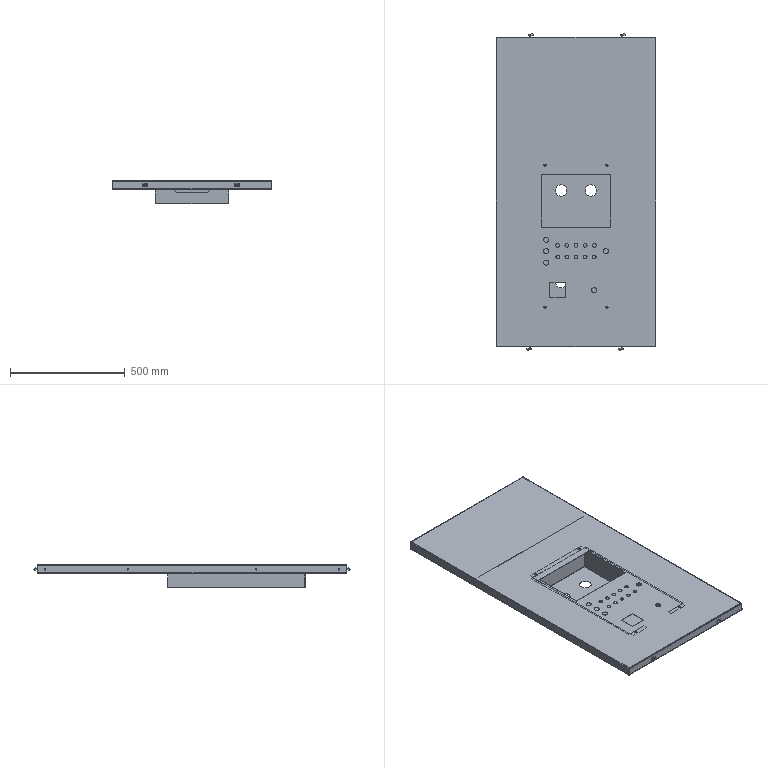Part | SolidWorks | features ReferencePattern 6, DerivedHolePattern 1 | 18 solids | 699 faces | box 697 x 1379 x 104.25 mm | volume 2244190 mm3 | plane 333 | cylinder 206 | cone 100 | spline 60 | commonest cylinder face diameters 20.854 x32 6.6 x24 16.2 x20 5.5 x16 1.6 x12 50 x12